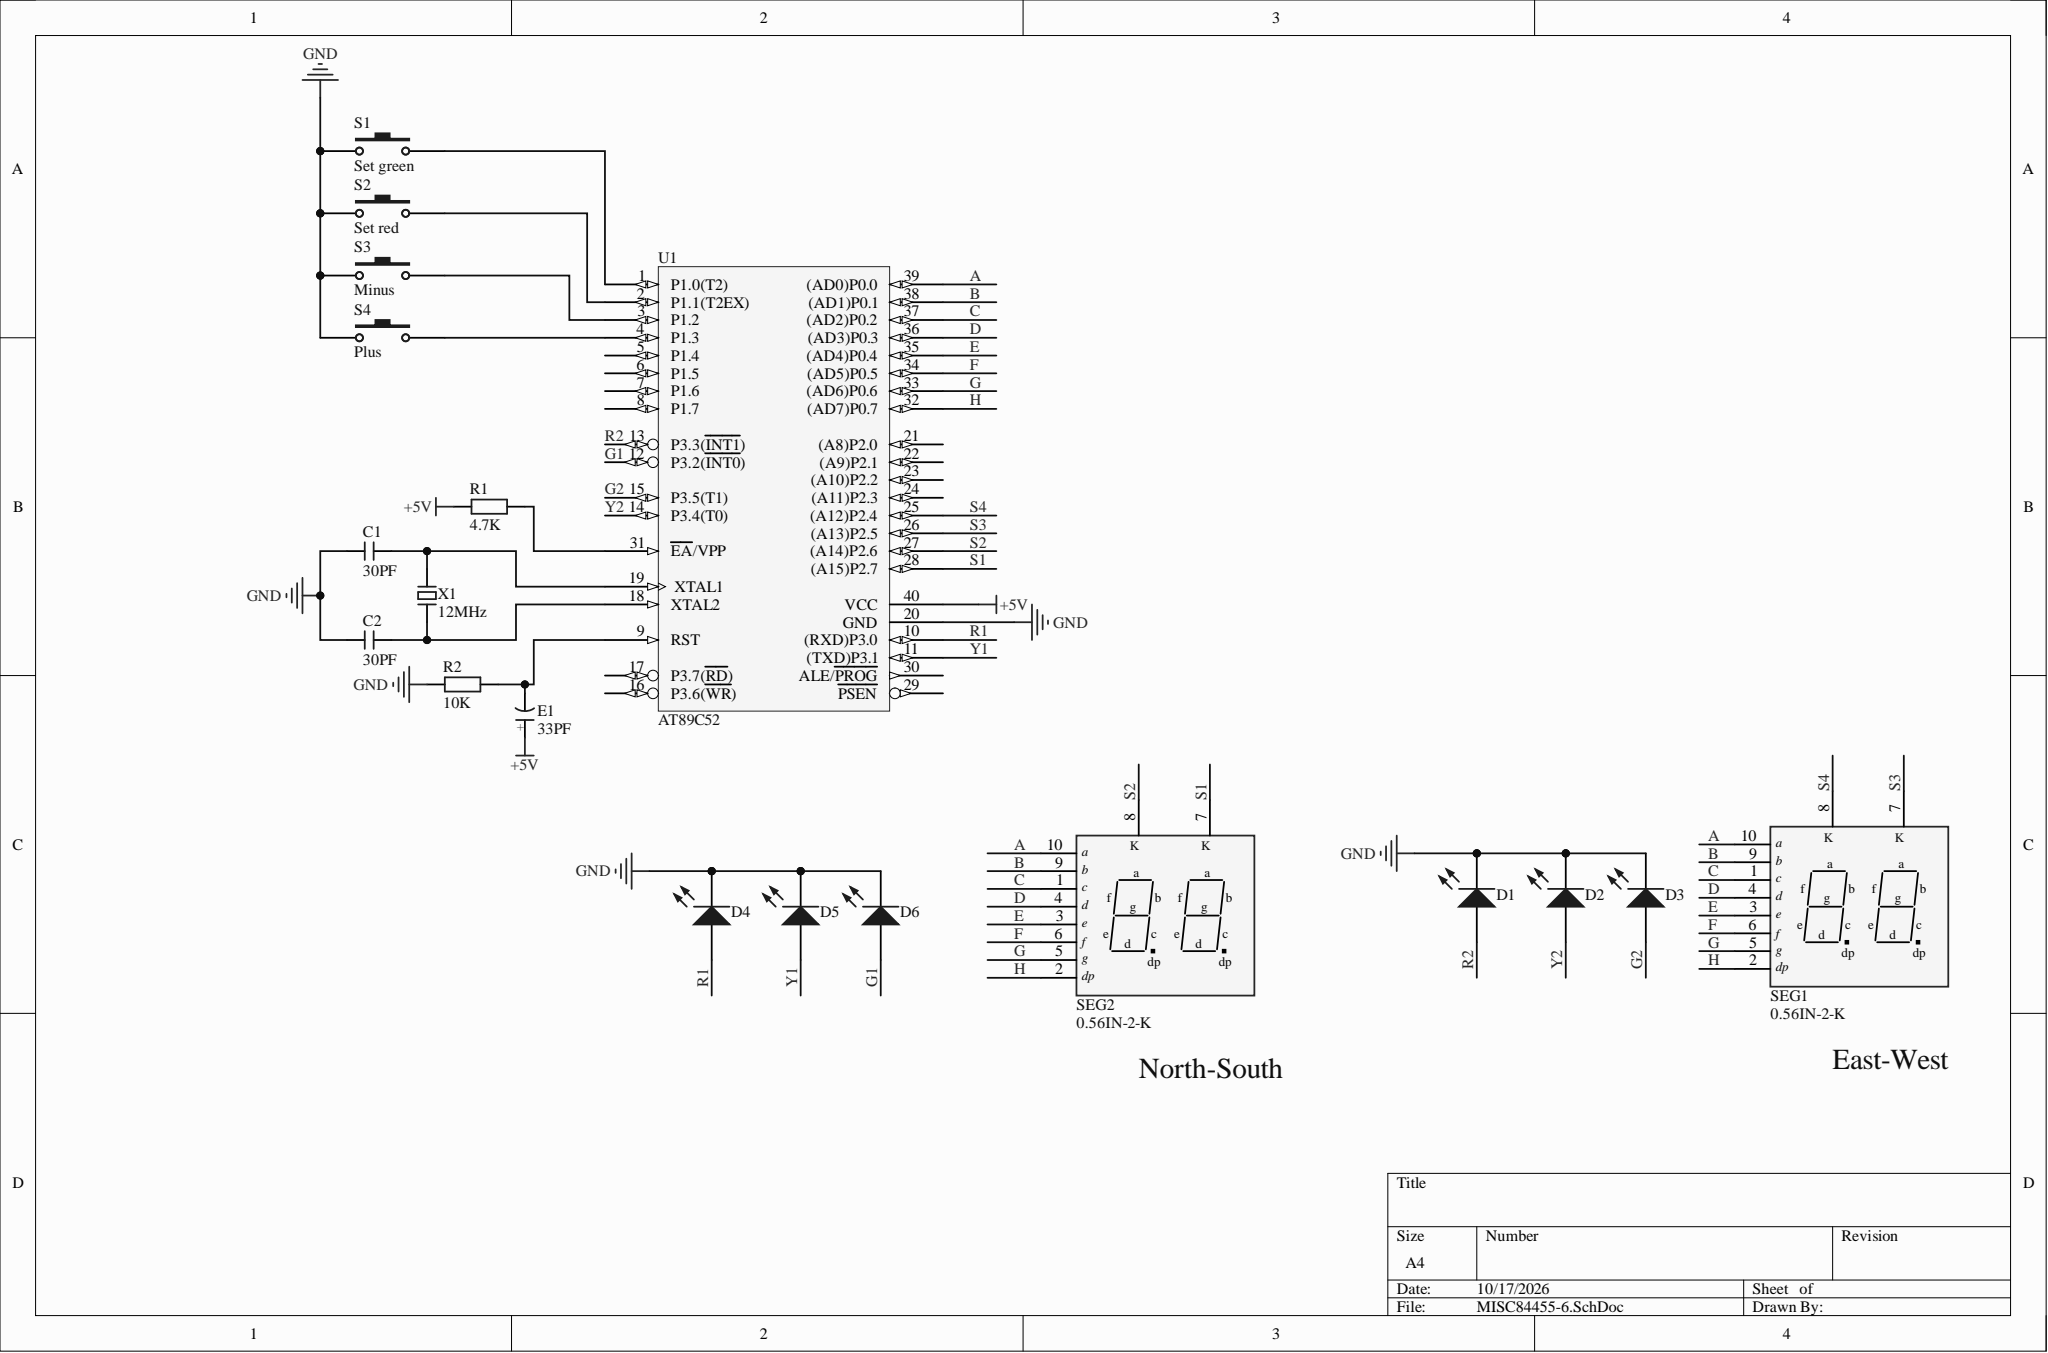Circuit board | Altium Designer | 19 parts | 28 nets
Bill of materials:
Comment,Description,Designator,Footprint,LibRef,Quantity
"30PF","ceramic disc capacitor","C1, C2","CC 1.8*3.6","CC","2"
"LED","light-emitting diode","D1, D2, D3, D4, D5, D6","LED 5MM-W","LED","6"
"33PF","through-hole solid-state capacitor","E1","CS 2.0*5*8 - C","CS","1"
"4.7K","colour-band resistor","R1","RS 1/4W","R-S","1"
"10K","colour-band resistor","R2","RS 1/4W","R-S","1"
"Set green","Switch","S1","四脚轻触开关","SW-PB","1"
"Set red","Switch","S2","四脚轻触开关","SW-PB","1"
"Minus","Switch","S3","四脚轻触开关","SW-PB","1"
"Plus","Switch","S4","四脚轻触开关","SW-PB","1"
"0.56IN-2-K","2-digit 0.56 inch common-cathode display","SEG1, SEG2","0.56IN-2P","0.56IN-2-K","2"
"AT89C52","","U1","DIP40","STC89C52","1"
"12MHz","2-pin passive crystal oscillator","X1","OSC HC-49S","XTAL-2P","1"
Netlist (Protel format):
[
C1
CC 1.8*3.6
30PF



]
[
C2
CC 1.8*3.6
30PF



]
[
D1
LED 5MM-W
LED



]
[
D2
LED 5MM-W
LED



]
[
D3
LED 5MM-W
LED



]
[
D4
LED 5MM-W
LED



]
[
D5
LED 5MM-W
LED



]
[
D6
LED 5MM-W
LED



]
[
E1
CS 2.0*5*8 - C
33PF



]
[
R1
RS 1/4W
4.7K



]
[
R2
RS 1/4W
10K



]
[
S1
四脚轻触开关
Set green



]
[
S2
四脚轻触开关
Set red



]
[
S3
四脚轻触开关
Minus



]
[
S4
四脚轻触开关
Plus



]
[
SEG1
0.56IN-2P
0.56IN-2-K



]
[
SEG2
0.56IN-2P
0.56IN-2-K



]
[
U1
DIP40
AT89C52



]
[
X1
OSC HC-49S
12MHz



]
(
Y2
D2-1
U1-14
)
(
Y1
D5-1
U1-11
)
(
S4
SEG1-8
U1-25
)
(
S3
SEG1-7
U1-26
)
(
S2
SEG2-8
U1-27
)
(
S1
SEG2-7
U1-28
)
(
R2
D1-1
U1-13
)
(
R1
D4-1
U1-10
)
(
NetS4_2
S4-2
U1-4
)
(
NetS3_2
S3-2
U1-3
)
(
NetS2_2
S2-2
U1-2
)
(
NetS1_2
S1-2
U1-1
)
(
NetR1_2
R1-2
U1-31
)
(
NetE1_2
E1-2
R2-2
U1-9
)
(
NetC2_2
C2-2
U1-18
X1-1
)
(
NetC1_2
C1-2
U1-19
X1-2
)
(
H
SEG1-2
SEG2-2
U1-32
)
(
GND
C1-1
C2-1
D1-2
D2-2
D3-2
D4-2
D5-2
D6-2
R2-1
S1-1
S2-1
S3-1
S4-1
U1-20
)
(
G2
D3-1
U1-15
)
(
G1
D6-1
U1-12
)
(
G
SEG1-5
SEG2-5
U1-33
)
(
F
SEG1-6
SEG2-6
U1-34
)
(
E
SEG1-3
SEG2-3
U1-35
)
(
D
SEG1-4
SEG2-4
U1-36
)
(
C
SEG1-1
SEG2-1
U1-37
)
(
B
SEG1-9
SEG2-9
U1-38
)
(
A
SEG1-10
SEG2-10
U1-39
)
(
+5V
E1-1
R1-1
U1-40
)